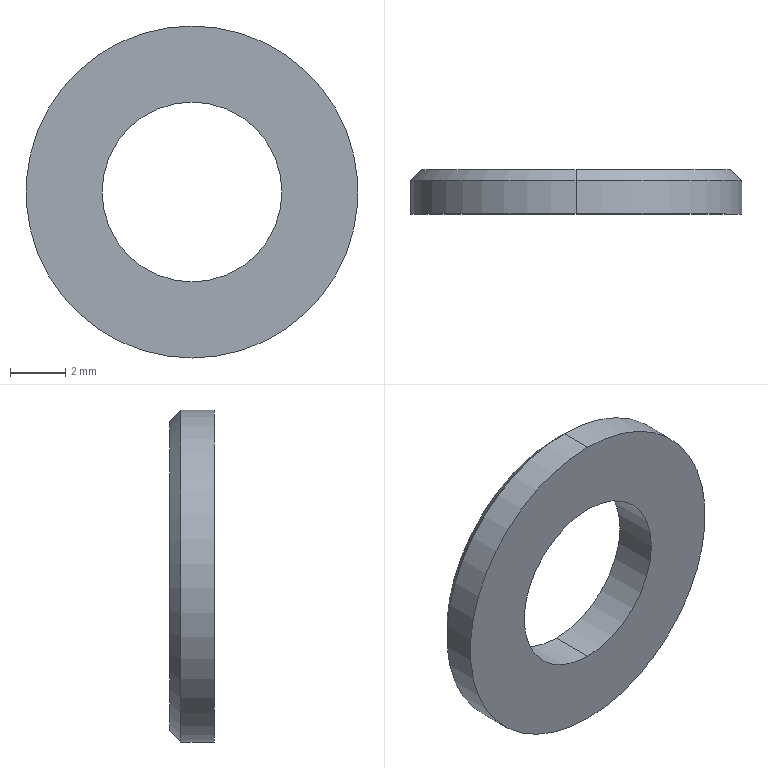Part | SolidWorks | features Chamfer 1, Extrusion 1 | 1 solid | 8 faces | box 12 x 1.6 x 12 mm | volume 124.914 mm3 | cylinder 4 | cone 2 | plane 2 | commonest cylinder face diameters 6.5 x2 12 x2
STEP:
#1=CARTESIAN_POINT('',(0.,1.6,5.6));
#2=VERTEX_POINT('',#1);
#3=CARTESIAN_POINT('',(0.,1.6,-5.6));
#4=VERTEX_POINT('',#3);
#5=CARTESIAN_POINT('',(0.,1.6,0.));
#6=DIRECTION('',(0.,1.,0.));
#7=DIRECTION('',(0.,0.,1.));
#8=AXIS2_PLACEMENT_3D('',#5,#6,#7);
#9=CIRCLE('',#8,5.6);
#10=EDGE_CURVE('',#2,#4,#9,.T.);
#11=ORIENTED_EDGE('',*,*,#10,.F.);
#12=CARTESIAN_POINT('',(0.,1.2,6.));
#13=VERTEX_POINT('',#12);
#14=CARTESIAN_POINT('',(0.,1.6,5.6));
#15=DIRECTION('',(0.,-0.7071,0.7071));
#16=VECTOR('',#15,1000.);
#17=LINE('',#14,#16);
#18=EDGE_CURVE('',#2,#13,#17,.T.);
#19=ORIENTED_EDGE('',*,*,#18,.T.);
#20=CARTESIAN_POINT('',(0.,1.2,-6.));
#21=VERTEX_POINT('',#20);
#22=CARTESIAN_POINT('',(0.,1.2,0.));
#23=DIRECTION('',(0.,-1.,0.));
#24=DIRECTION('',(0.,0.,1.));
#25=AXIS2_PLACEMENT_3D('',#22,#23,#24);
#26=CIRCLE('',#25,6.);
#27=EDGE_CURVE('',#21,#13,#26,.T.);
#28=ORIENTED_EDGE('',*,*,#27,.F.);
#29=CARTESIAN_POINT('',(0.,1.6,-5.6));
#30=DIRECTION('',(0.,-0.7071,-0.7071));
#31=VECTOR('',#30,1000.);
#32=LINE('',#29,#31);
#33=EDGE_CURVE('',#4,#21,#32,.T.);
#34=ORIENTED_EDGE('',*,*,#33,.F.);
#35=EDGE_LOOP('',(#11,#19,#28,#34));
#36=FACE_OUTER_BOUND('',#35,.T.);
#37=CARTESIAN_POINT('',(0.,1.6,0.));
#38=DIRECTION('',(0.,-1.,0.));
#39=DIRECTION('',(0.,0.,-1.));
#40=AXIS2_PLACEMENT_3D('',#37,#38,#39);
#41=CONICAL_SURFACE('',#40,5.6,0.7854);
#42=ADVANCED_FACE('',(#36),#41,.T.);
#43=CARTESIAN_POINT('',(0.,1.6,-3.25));
#44=VERTEX_POINT('',#43);
#45=CARTESIAN_POINT('',(0.,1.6,3.25));
#46=VERTEX_POINT('',#45);
#47=CARTESIAN_POINT('',(0.,1.6,0.));
#48=DIRECTION('',(0.,1.,0.));
#49=DIRECTION('',(0.,0.,1.));
#50=AXIS2_PLACEMENT_3D('',#47,#48,#49);
#51=CIRCLE('',#50,3.25);
#52=EDGE_CURVE('',#44,#46,#51,.T.);
#53=ORIENTED_EDGE('',*,*,#52,.T.);
#54=CARTESIAN_POINT('',(0.,0.,3.25));
#55=VERTEX_POINT('',#54);
#56=CARTESIAN_POINT('',(0.,1.6,3.25));
#57=DIRECTION('',(0.,-1.,0.));
#58=VECTOR('',#57,1000.);
#59=LINE('',#56,#58);
#60=EDGE_CURVE('',#46,#55,#59,.T.);
#61=ORIENTED_EDGE('',*,*,#60,.T.);
#62=CARTESIAN_POINT('',(0.,0.,-3.25));
#63=VERTEX_POINT('',#62);
#64=CARTESIAN_POINT('',(0.,0.,0.));
#65=DIRECTION('',(0.,1.,0.));
#66=DIRECTION('',(0.,0.,1.));
#67=AXIS2_PLACEMENT_3D('',#64,#65,#66);
#68=CIRCLE('',#67,3.25);
#69=EDGE_CURVE('',#63,#55,#68,.T.);
#70=ORIENTED_EDGE('',*,*,#69,.F.);
#71=CARTESIAN_POINT('',(0.,1.6,-3.25));
#72=DIRECTION('',(0.,-1.,0.));
#73=VECTOR('',#72,1000.);
#74=LINE('',#71,#73);
#75=EDGE_CURVE('',#44,#63,#74,.T.);
#76=ORIENTED_EDGE('',*,*,#75,.F.);
#77=EDGE_LOOP('',(#53,#61,#70,#76));
#78=FACE_OUTER_BOUND('',#77,.T.);
#79=CARTESIAN_POINT('',(0.,1.6,0.));
#80=DIRECTION('',(0.,-1.,0.));
#81=DIRECTION('',(0.,0.,-1.));
#82=AXIS2_PLACEMENT_3D('',#79,#80,#81);
#83=CYLINDRICAL_SURFACE('',#82,3.25);
#84=ADVANCED_FACE('',(#78),#83,.F.);
#85=ORIENTED_EDGE('',*,*,#27,.T.);
#86=CARTESIAN_POINT('',(0.,0.,6.));
#87=VERTEX_POINT('',#86);
#88=CARTESIAN_POINT('',(0.,1.6,6.));
#89=DIRECTION('',(0.,-1.,0.));
#90=VECTOR('',#89,1000.);
#91=LINE('',#88,#90);
#92=EDGE_CURVE('',#13,#87,#91,.T.);
#93=ORIENTED_EDGE('',*,*,#92,.T.);
#94=CARTESIAN_POINT('',(0.,0.,-6.));
#95=VERTEX_POINT('',#94);
#96=CARTESIAN_POINT('',(0.,0.,0.));
#97=DIRECTION('',(0.,1.,0.));
#98=DIRECTION('',(0.,0.,1.));
#99=AXIS2_PLACEMENT_3D('',#96,#97,#98);
#100=CIRCLE('',#99,6.);
#101=EDGE_CURVE('',#87,#95,#100,.T.);
#102=ORIENTED_EDGE('',*,*,#101,.T.);
#103=CARTESIAN_POINT('',(0.,1.6,-6.));
#104=DIRECTION('',(0.,-1.,0.));
#105=VECTOR('',#104,1000.);
#106=LINE('',#103,#105);
#107=EDGE_CURVE('',#21,#95,#106,.T.);
#108=ORIENTED_EDGE('',*,*,#107,.F.);
#109=EDGE_LOOP('',(#85,#93,#102,#108));
#110=FACE_OUTER_BOUND('',#109,.T.);
#111=CARTESIAN_POINT('',(0.,1.6,0.));
#112=DIRECTION('',(0.,-1.,0.));
#113=DIRECTION('',(0.,0.,-1.));
#114=AXIS2_PLACEMENT_3D('',#111,#112,#113);
#115=CYLINDRICAL_SURFACE('',#114,6.);
#116=ADVANCED_FACE('',(#110),#115,.T.);
#117=CARTESIAN_POINT('',(0.,1.6,0.));
#118=DIRECTION('',(0.,1.,0.));
#119=DIRECTION('',(0.,0.,1.));
#120=AXIS2_PLACEMENT_3D('',#117,#118,#119);
#121=CIRCLE('',#120,5.6);
#122=EDGE_CURVE('',#4,#2,#121,.T.);
#123=ORIENTED_EDGE('',*,*,#122,.T.);
#124=ORIENTED_EDGE('',*,*,#10,.T.);
#125=EDGE_LOOP('',(#123,#124));
#126=FACE_OUTER_BOUND('',#125,.T.);
#127=ORIENTED_EDGE('',*,*,#52,.F.);
#128=CARTESIAN_POINT('',(0.,1.6,0.));
#129=DIRECTION('',(0.,1.,0.));
#130=DIRECTION('',(0.,0.,1.));
#131=AXIS2_PLACEMENT_3D('',#128,#129,#130);
#132=CIRCLE('',#131,3.25);
#133=EDGE_CURVE('',#46,#44,#132,.T.);
#134=ORIENTED_EDGE('',*,*,#133,.F.);
#135=EDGE_LOOP('',(#127,#134));
#136=FACE_BOUND('',#135,.T.);
#137=CARTESIAN_POINT('',(0.,1.6,0.));
#138=DIRECTION('',(0.,1.,0.));
#139=DIRECTION('',(0.,0.,1.));
#140=AXIS2_PLACEMENT_3D('',#137,#138,#139);
#141=PLANE('',#140);
#142=ADVANCED_FACE('',(#126,#136),#141,.T.);
#143=CARTESIAN_POINT('',(0.,0.,0.));
#144=DIRECTION('',(0.,1.,0.));
#145=DIRECTION('',(0.,0.,1.));
#146=AXIS2_PLACEMENT_3D('',#143,#144,#145);
#147=CIRCLE('',#146,6.);
#148=EDGE_CURVE('',#95,#87,#147,.T.);
#149=ORIENTED_EDGE('',*,*,#148,.F.);
#150=ORIENTED_EDGE('',*,*,#101,.F.);
#151=EDGE_LOOP('',(#149,#150));
#152=FACE_OUTER_BOUND('',#151,.T.);
#153=ORIENTED_EDGE('',*,*,#69,.T.);
#154=CARTESIAN_POINT('',(0.,0.,0.));
#155=DIRECTION('',(0.,1.,0.));
#156=DIRECTION('',(0.,0.,1.));
#157=AXIS2_PLACEMENT_3D('',#154,#155,#156);
#158=CIRCLE('',#157,3.25);
#159=EDGE_CURVE('',#55,#63,#158,.T.);
#160=ORIENTED_EDGE('',*,*,#159,.T.);
#161=EDGE_LOOP('',(#153,#160));
#162=FACE_BOUND('',#161,.T.);
#163=CARTESIAN_POINT('',(0.,0.,0.));
#164=DIRECTION('',(0.,1.,0.));
#165=DIRECTION('',(0.,0.,1.));
#166=AXIS2_PLACEMENT_3D('',#163,#164,#165);
#167=PLANE('',#166);
#168=ADVANCED_FACE('',(#152,#162),#167,.F.);
#169=ORIENTED_EDGE('',*,*,#92,.F.);
#170=CARTESIAN_POINT('',(0.,1.2,0.));
#171=DIRECTION('',(0.,-1.,0.));
#172=DIRECTION('',(0.,0.,1.));
#173=AXIS2_PLACEMENT_3D('',#170,#171,#172);
#174=CIRCLE('',#173,6.);
#175=EDGE_CURVE('',#13,#21,#174,.T.);
#176=ORIENTED_EDGE('',*,*,#175,.T.);
#177=ORIENTED_EDGE('',*,*,#107,.T.);
#178=ORIENTED_EDGE('',*,*,#148,.T.);
#179=EDGE_LOOP('',(#169,#176,#177,#178));
#180=FACE_OUTER_BOUND('',#179,.T.);
#181=CARTESIAN_POINT('',(0.,1.6,0.));
#182=DIRECTION('',(0.,-1.,0.));
#183=DIRECTION('',(0.,0.,-1.));
#184=AXIS2_PLACEMENT_3D('',#181,#182,#183);
#185=CYLINDRICAL_SURFACE('',#184,6.);
#186=ADVANCED_FACE('',(#180),#185,.T.);
#187=ORIENTED_EDGE('',*,*,#60,.F.);
#188=ORIENTED_EDGE('',*,*,#133,.T.);
#189=ORIENTED_EDGE('',*,*,#75,.T.);
#190=ORIENTED_EDGE('',*,*,#159,.F.);
#191=EDGE_LOOP('',(#187,#188,#189,#190));
#192=FACE_OUTER_BOUND('',#191,.T.);
#193=CARTESIAN_POINT('',(0.,1.6,0.));
#194=DIRECTION('',(0.,-1.,0.));
#195=DIRECTION('',(0.,0.,-1.));
#196=AXIS2_PLACEMENT_3D('',#193,#194,#195);
#197=CYLINDRICAL_SURFACE('',#196,3.25);
#198=ADVANCED_FACE('',(#192),#197,.F.);
#199=ORIENTED_EDGE('',*,*,#18,.F.);
#200=ORIENTED_EDGE('',*,*,#122,.F.);
#201=ORIENTED_EDGE('',*,*,#33,.T.);
#202=ORIENTED_EDGE('',*,*,#175,.F.);
#203=EDGE_LOOP('',(#199,#200,#201,#202));
#204=FACE_OUTER_BOUND('',#203,.T.);
#205=CARTESIAN_POINT('',(0.,1.6,0.));
#206=DIRECTION('',(0.,-1.,0.));
#207=DIRECTION('',(0.,0.,-1.));
#208=AXIS2_PLACEMENT_3D('',#205,#206,#207);
#209=CONICAL_SURFACE('',#208,5.6,0.7854);
#210=ADVANCED_FACE('',(#204),#209,.T.);
#211=CLOSED_SHELL('',(#42,#84,#116,#142,#168,#186,#198,#210));
#212=MANIFOLD_SOLID_BREP('',#211);
#213=CARTESIAN_POINT('',(0.,0.,0.));
#214=DIRECTION('',(0.,0.,1.));
#215=DIRECTION('',(1.,0.,0.));
#216=AXIS2_PLACEMENT_3D('',#213,#214,#215);
#217=(LENGTH_UNIT()NAMED_UNIT(*)SI_UNIT(.MILLI.,.METRE.));
#218=UNCERTAINTY_MEASURE_WITH_UNIT(LENGTH_MEASURE(0.00001),#217,'','');
#219=(NAMED_UNIT(*)PLANE_ANGLE_UNIT()SI_UNIT($,.RADIAN.));
#220=(NAMED_UNIT(*)SI_UNIT($,.STERADIAN.)SOLID_ANGLE_UNIT());
#221=(GEOMETRIC_REPRESENTATION_CONTEXT(3)GLOBAL_UNCERTAINTY_ASSIGNED_CONTEXT((#218))GLOBAL_UNIT_ASSIGNED_CONTEXT((#217,#219,#220))REPRESENTATION_CONTEXT('',''));
#222=ADVANCED_BREP_SHAPE_REPRESENTATION('',(#212,#216),#221);